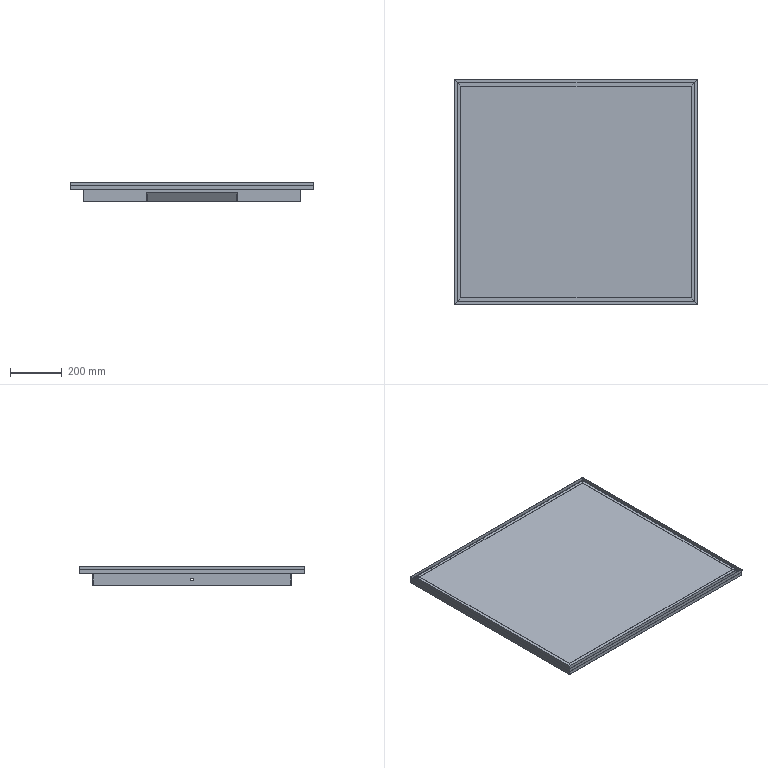Part | 7 solids | 282 faces | box 940 x 870 x 75 mm | volume 17902552 mm3 | plane 148 | cylinder 122 | spline 12 | commonest cylinder face diameters 4.2 x80 11 x14 0.4 x11 2.4 x11 10 x6